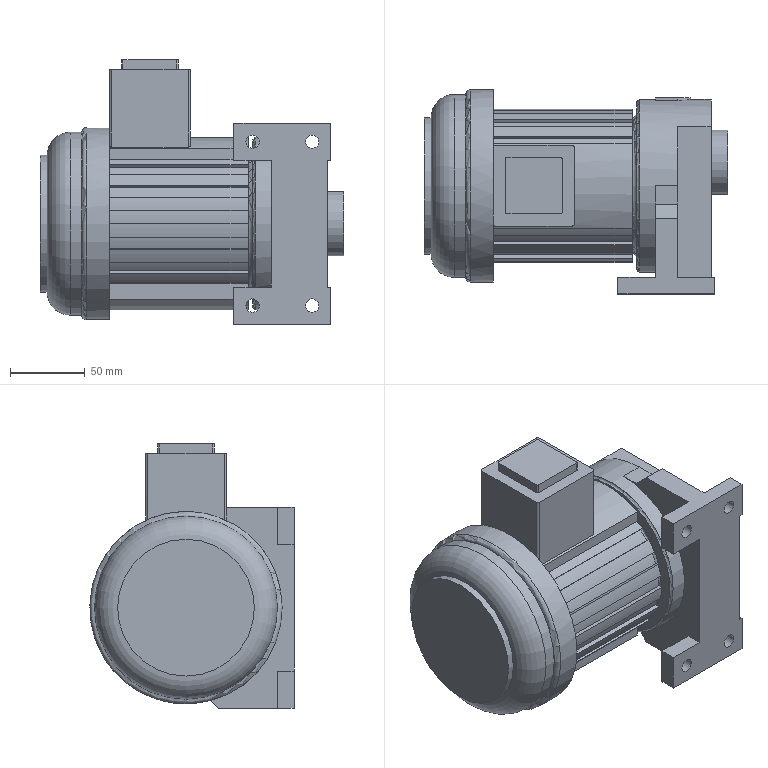Part | STEP file | basic_gh_motor_gh1_02 | 1 solid | 118 faces | box 203.75 x 137 x 177.5 mm | volume 2157267 mm3 | plane 70 | cylinder 44 | torus 4 | commonest cylinder face diameters 98.04 x12 103.2 x12 1.806 x4 2.58 x4 9 x4 116.1 x2